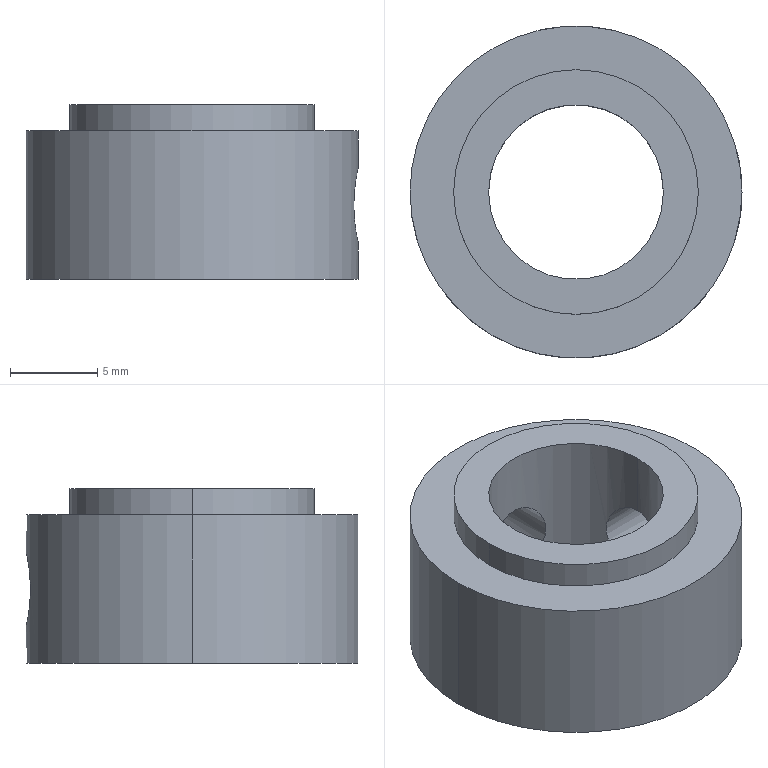Part | STEP file | 602-03-0014 | 1 solid | 13 faces | box 19 x 19 x 10 mm | volume 1729 mm3 | cylinder 10 | plane 3 | commonest cylinder face diameters 4.2 x4 10 x2 14 x2 19 x2